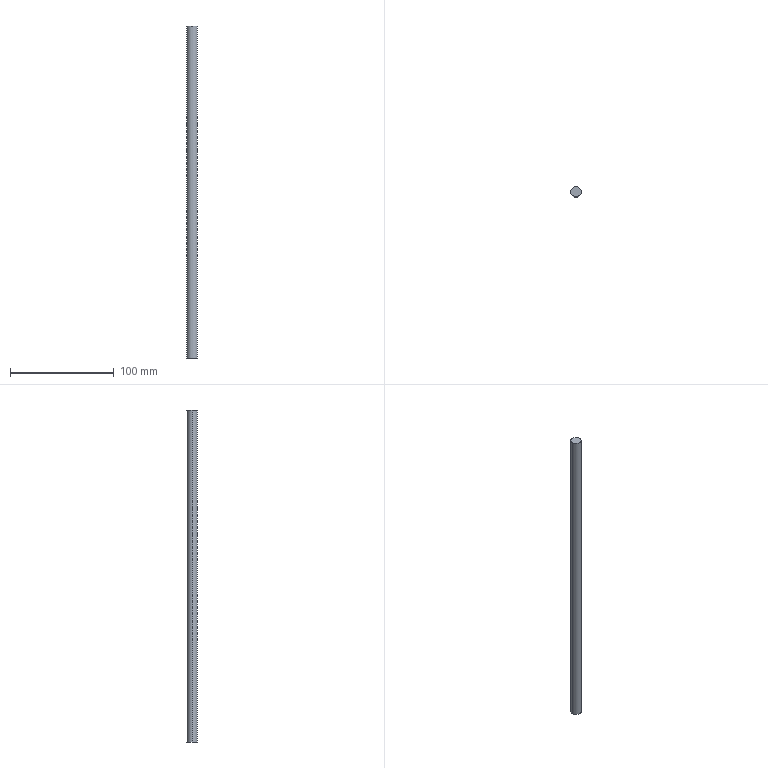Part | SolidWorks | features Extrusion 1 | 1 solid | 4 faces | box 10 x 10 x 320 mm | volume 25133 mm3 | cylinder 2 | plane 2 | commonest cylinder face diameters 10 x2
STEP:
#1=CARTESIAN_POINT('',(5.,0.,320.));
#2=VERTEX_POINT('',#1);
#3=CARTESIAN_POINT('',(-5.,0.,320.));
#4=VERTEX_POINT('',#3);
#5=CARTESIAN_POINT('',(0.,0.,320.));
#6=DIRECTION('',(0.,0.,1.));
#7=DIRECTION('',(1.,0.,0.));
#8=AXIS2_PLACEMENT_3D('',#5,#6,#7);
#9=CIRCLE('',#8,5.);
#10=EDGE_CURVE('',#2,#4,#9,.T.);
#11=ORIENTED_EDGE('',*,*,#10,.F.);
#12=CARTESIAN_POINT('',(5.,0.,0.));
#13=VERTEX_POINT('',#12);
#14=CARTESIAN_POINT('',(5.,0.,320.));
#15=DIRECTION('',(0.,0.,-1.));
#16=VECTOR('',#15,1000.);
#17=LINE('',#14,#16);
#18=EDGE_CURVE('',#2,#13,#17,.T.);
#19=ORIENTED_EDGE('',*,*,#18,.T.);
#20=CARTESIAN_POINT('',(-5.,0.,0.));
#21=VERTEX_POINT('',#20);
#22=CARTESIAN_POINT('',(0.,0.,0.));
#23=DIRECTION('',(0.,0.,1.));
#24=DIRECTION('',(1.,0.,0.));
#25=AXIS2_PLACEMENT_3D('',#22,#23,#24);
#26=CIRCLE('',#25,5.);
#27=EDGE_CURVE('',#13,#21,#26,.T.);
#28=ORIENTED_EDGE('',*,*,#27,.T.);
#29=CARTESIAN_POINT('',(-5.,0.,320.));
#30=DIRECTION('',(0.,0.,-1.));
#31=VECTOR('',#30,1000.);
#32=LINE('',#29,#31);
#33=EDGE_CURVE('',#4,#21,#32,.T.);
#34=ORIENTED_EDGE('',*,*,#33,.F.);
#35=EDGE_LOOP('',(#11,#19,#28,#34));
#36=FACE_OUTER_BOUND('',#35,.T.);
#37=CARTESIAN_POINT('',(0.,0.,320.));
#38=DIRECTION('',(0.,0.,-1.));
#39=DIRECTION('',(-1.,0.,0.));
#40=AXIS2_PLACEMENT_3D('',#37,#38,#39);
#41=CYLINDRICAL_SURFACE('',#40,5.);
#42=ADVANCED_FACE('',(#36),#41,.T.);
#43=ORIENTED_EDGE('',*,*,#18,.F.);
#44=CARTESIAN_POINT('',(0.,0.,320.));
#45=DIRECTION('',(0.,0.,1.));
#46=DIRECTION('',(1.,0.,0.));
#47=AXIS2_PLACEMENT_3D('',#44,#45,#46);
#48=CIRCLE('',#47,5.);
#49=EDGE_CURVE('',#4,#2,#48,.T.);
#50=ORIENTED_EDGE('',*,*,#49,.F.);
#51=ORIENTED_EDGE('',*,*,#33,.T.);
#52=CARTESIAN_POINT('',(0.,0.,0.));
#53=DIRECTION('',(0.,0.,1.));
#54=DIRECTION('',(1.,0.,0.));
#55=AXIS2_PLACEMENT_3D('',#52,#53,#54);
#56=CIRCLE('',#55,5.);
#57=EDGE_CURVE('',#21,#13,#56,.T.);
#58=ORIENTED_EDGE('',*,*,#57,.T.);
#59=EDGE_LOOP('',(#43,#50,#51,#58));
#60=FACE_OUTER_BOUND('',#59,.T.);
#61=CARTESIAN_POINT('',(0.,0.,320.));
#62=DIRECTION('',(0.,0.,-1.));
#63=DIRECTION('',(-1.,0.,0.));
#64=AXIS2_PLACEMENT_3D('',#61,#62,#63);
#65=CYLINDRICAL_SURFACE('',#64,5.);
#66=ADVANCED_FACE('',(#60),#65,.T.);
#67=ORIENTED_EDGE('',*,*,#49,.T.);
#68=ORIENTED_EDGE('',*,*,#10,.T.);
#69=EDGE_LOOP('',(#67,#68));
#70=FACE_OUTER_BOUND('',#69,.T.);
#71=CARTESIAN_POINT('',(0.,0.,320.));
#72=DIRECTION('',(0.,0.,1.));
#73=DIRECTION('',(1.,0.,0.));
#74=AXIS2_PLACEMENT_3D('',#71,#72,#73);
#75=PLANE('',#74);
#76=ADVANCED_FACE('',(#70),#75,.T.);
#77=ORIENTED_EDGE('',*,*,#57,.F.);
#78=ORIENTED_EDGE('',*,*,#27,.F.);
#79=EDGE_LOOP('',(#77,#78));
#80=FACE_OUTER_BOUND('',#79,.T.);
#81=CARTESIAN_POINT('',(0.,0.,0.));
#82=DIRECTION('',(0.,0.,1.));
#83=DIRECTION('',(1.,0.,0.));
#84=AXIS2_PLACEMENT_3D('',#81,#82,#83);
#85=PLANE('',#84);
#86=ADVANCED_FACE('',(#80),#85,.F.);
#87=CLOSED_SHELL('',(#42,#66,#76,#86));
#88=MANIFOLD_SOLID_BREP('',#87);
#89=CARTESIAN_POINT('',(0.,0.,0.));
#90=DIRECTION('',(0.,0.,1.));
#91=DIRECTION('',(1.,0.,0.));
#92=AXIS2_PLACEMENT_3D('',#89,#90,#91);
#93=(LENGTH_UNIT()NAMED_UNIT(*)SI_UNIT(.MILLI.,.METRE.));
#94=UNCERTAINTY_MEASURE_WITH_UNIT(LENGTH_MEASURE(0.00001),#93,'','');
#95=(NAMED_UNIT(*)PLANE_ANGLE_UNIT()SI_UNIT($,.RADIAN.));
#96=(NAMED_UNIT(*)SI_UNIT($,.STERADIAN.)SOLID_ANGLE_UNIT());
#97=(GEOMETRIC_REPRESENTATION_CONTEXT(3)GLOBAL_UNCERTAINTY_ASSIGNED_CONTEXT((#94))GLOBAL_UNIT_ASSIGNED_CONTEXT((#93,#95,#96))REPRESENTATION_CONTEXT('',''));
#98=ADVANCED_BREP_SHAPE_REPRESENTATION('',(#88,#92),#97);